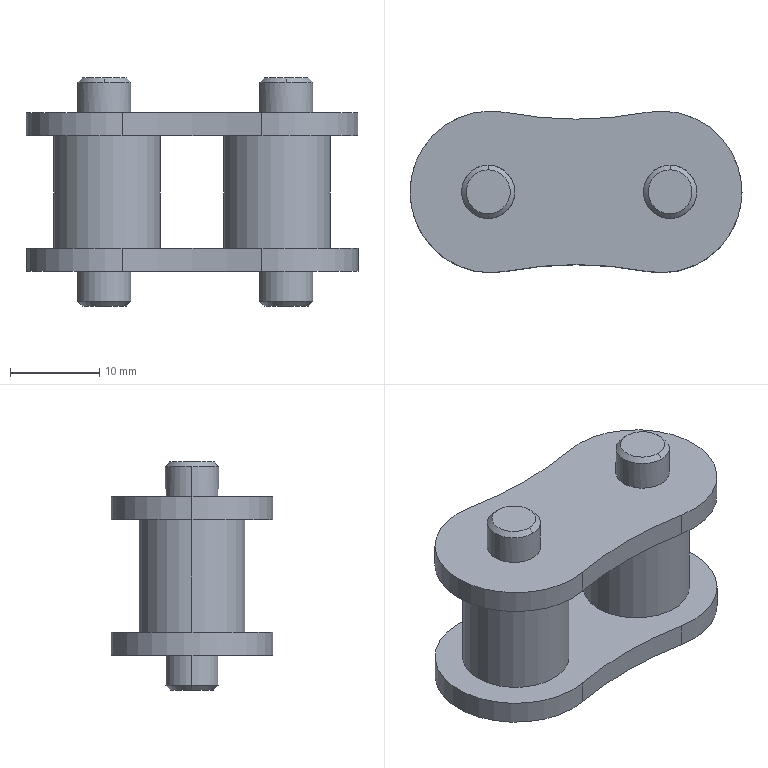Part | SolidWorks | features MoveFace 2, BaseBody 1 | 1 solid | 38 faces | box 37.13 x 18.08 x 25.52 mm | volume 6230 mm3 | cylinder 22 | cone 8 | plane 8 | commonest cylinder face diameters 5.96 x8 18.08 x6 11.91 x4 83.184 x4
STEP:
#1=CARTESIAN_POINT('',(-85.67,-121.776,-8.875));
#2=VERTEX_POINT('',#1);
#3=CARTESIAN_POINT('',(-96.411,-130.655,-8.875));
#4=VERTEX_POINT('',#3);
#5=CARTESIAN_POINT('',(-94.71,-121.776,-8.875));
#6=DIRECTION('',(0.,0.,-1.));
#7=DIRECTION('',(1.,0.,0.));
#8=AXIS2_PLACEMENT_3D('',#5,#6,#7);
#9=CIRCLE('',#8,9.04);
#10=EDGE_CURVE('',#2,#4,#9,.T.);
#11=ORIENTED_EDGE('',*,*,#10,.F.);
#12=CARTESIAN_POINT('',(-85.67,-121.776,-6.285));
#13=VERTEX_POINT('',#12);
#14=CARTESIAN_POINT('',(-85.67,-121.776,-8.875));
#15=DIRECTION('',(0.,0.,1.));
#16=VECTOR('',#15,1000.);
#17=LINE('',#14,#16);
#18=EDGE_CURVE('',#2,#13,#17,.T.);
#19=ORIENTED_EDGE('',*,*,#18,.T.);
#20=CARTESIAN_POINT('',(-96.411,-130.655,-6.285));
#21=VERTEX_POINT('',#20);
#22=CARTESIAN_POINT('',(-94.71,-121.776,-6.285));
#23=DIRECTION('',(0.,0.,-1.));
#24=DIRECTION('',(1.,0.,0.));
#25=AXIS2_PLACEMENT_3D('',#22,#23,#24);
#26=CIRCLE('',#25,9.04);
#27=EDGE_CURVE('',#13,#21,#26,.T.);
#28=ORIENTED_EDGE('',*,*,#27,.T.);
#29=CARTESIAN_POINT('',(-96.411,-130.655,-8.875));
#30=DIRECTION('',(0.,0.,-1.));
#31=VECTOR('',#30,1000.);
#32=LINE('',#29,#31);
#33=EDGE_CURVE('',#21,#4,#32,.T.);
#34=ORIENTED_EDGE('',*,*,#33,.T.);
#35=EDGE_LOOP('',(#11,#19,#28,#34));
#36=FACE_OUTER_BOUND('',#35,.T.);
#37=CARTESIAN_POINT('',(-94.71,-121.776,-8.875));
#38=DIRECTION('',(0.,0.,1.));
#39=DIRECTION('',(1.,0.,0.));
#40=AXIS2_PLACEMENT_3D('',#37,#38,#39);
#41=CYLINDRICAL_SURFACE('',#40,9.04);
#42=ADVANCED_FACE('',(#36),#41,.T.);
#43=CARTESIAN_POINT('',(-111.08,-121.776,-12.242));
#44=VERTEX_POINT('',#43);
#45=CARTESIAN_POINT('',(-117.04,-121.776,-12.242));
#46=VERTEX_POINT('',#45);
#47=CARTESIAN_POINT('',(-114.06,-121.776,-12.242));
#48=DIRECTION('',(0.,0.,1.));
#49=DIRECTION('',(1.,0.,0.));
#50=AXIS2_PLACEMENT_3D('',#47,#48,#49);
#51=CIRCLE('',#50,2.98);
#52=EDGE_CURVE('',#44,#46,#51,.T.);
#53=ORIENTED_EDGE('',*,*,#52,.T.);
#54=CARTESIAN_POINT('',(-117.04,-121.776,-8.875));
#55=VERTEX_POINT('',#54);
#56=CARTESIAN_POINT('',(-117.04,-121.776,-12.76));
#57=DIRECTION('',(0.,0.,1.));
#58=VECTOR('',#57,1000.);
#59=LINE('',#56,#58);
#60=EDGE_CURVE('',#46,#55,#59,.T.);
#61=ORIENTED_EDGE('',*,*,#60,.T.);
#62=CARTESIAN_POINT('',(-111.08,-121.776,-8.875));
#63=VERTEX_POINT('',#62);
#64=CARTESIAN_POINT('',(-114.06,-121.776,-8.875));
#65=DIRECTION('',(0.,0.,1.));
#66=DIRECTION('',(1.,0.,0.));
#67=AXIS2_PLACEMENT_3D('',#64,#65,#66);
#68=CIRCLE('',#67,2.98);
#69=EDGE_CURVE('',#63,#55,#68,.T.);
#70=ORIENTED_EDGE('',*,*,#69,.F.);
#71=CARTESIAN_POINT('',(-111.08,-121.776,-12.76));
#72=DIRECTION('',(0.,0.,1.));
#73=VECTOR('',#72,1000.);
#74=LINE('',#71,#73);
#75=EDGE_CURVE('',#44,#63,#74,.T.);
#76=ORIENTED_EDGE('',*,*,#75,.F.);
#77=EDGE_LOOP('',(#53,#61,#70,#76));
#78=FACE_OUTER_BOUND('',#77,.T.);
#79=CARTESIAN_POINT('',(-114.06,-121.776,-12.76));
#80=DIRECTION('',(0.,0.,1.));
#81=DIRECTION('',(1.,0.,0.));
#82=AXIS2_PLACEMENT_3D('',#79,#80,#81);
#83=CYLINDRICAL_SURFACE('',#82,2.98);
#84=ADVANCED_FACE('',(#78),#83,.T.);
#85=CARTESIAN_POINT('',(-90.73,-121.776,-12.242));
#86=VERTEX_POINT('',#85);
#87=CARTESIAN_POINT('',(-96.69,-121.776,-12.242));
#88=VERTEX_POINT('',#87);
#89=CARTESIAN_POINT('',(-93.71,-121.776,-12.242));
#90=DIRECTION('',(0.,0.,1.));
#91=DIRECTION('',(1.,0.,0.));
#92=AXIS2_PLACEMENT_3D('',#89,#90,#91);
#93=CIRCLE('',#92,2.98);
#94=EDGE_CURVE('',#86,#88,#93,.T.);
#95=ORIENTED_EDGE('',*,*,#94,.T.);
#96=CARTESIAN_POINT('',(-96.69,-121.776,-8.875));
#97=VERTEX_POINT('',#96);
#98=CARTESIAN_POINT('',(-96.69,-121.776,-12.76));
#99=DIRECTION('',(0.,0.,1.));
#100=VECTOR('',#99,1000.);
#101=LINE('',#98,#100);
#102=EDGE_CURVE('',#88,#97,#101,.T.);
#103=ORIENTED_EDGE('',*,*,#102,.T.);
#104=CARTESIAN_POINT('',(-90.73,-121.776,-8.875));
#105=VERTEX_POINT('',#104);
#106=CARTESIAN_POINT('',(-93.71,-121.776,-8.875));
#107=DIRECTION('',(0.,0.,1.));
#108=DIRECTION('',(1.,0.,0.));
#109=AXIS2_PLACEMENT_3D('',#106,#107,#108);
#110=CIRCLE('',#109,2.98);
#111=EDGE_CURVE('',#105,#97,#110,.T.);
#112=ORIENTED_EDGE('',*,*,#111,.F.);
#113=CARTESIAN_POINT('',(-90.73,-121.776,-12.76));
#114=DIRECTION('',(0.,0.,1.));
#115=VECTOR('',#114,1000.);
#116=LINE('',#113,#115);
#117=EDGE_CURVE('',#86,#105,#116,.T.);
#118=ORIENTED_EDGE('',*,*,#117,.F.);
#119=EDGE_LOOP('',(#95,#103,#112,#118));
#120=FACE_OUTER_BOUND('',#119,.T.);
#121=CARTESIAN_POINT('',(-93.71,-121.776,-12.76));
#122=DIRECTION('',(0.,0.,1.));
#123=DIRECTION('',(1.,0.,0.));
#124=AXIS2_PLACEMENT_3D('',#121,#122,#123);
#125=CYLINDRICAL_SURFACE('',#124,2.98);
#126=ADVANCED_FACE('',(#120),#125,.T.);
#127=CARTESIAN_POINT('',(-111.598,-121.776,-12.76));
#128=VERTEX_POINT('',#127);
#129=CARTESIAN_POINT('',(-116.522,-121.776,-12.76));
#130=VERTEX_POINT('',#129);
#131=CARTESIAN_POINT('',(-114.06,-121.776,-12.76));
#132=DIRECTION('',(0.,0.,1.));
#133=DIRECTION('',(1.,0.,0.));
#134=AXIS2_PLACEMENT_3D('',#131,#132,#133);
#135=CIRCLE('',#134,2.462);
#136=EDGE_CURVE('',#128,#130,#135,.T.);
#137=ORIENTED_EDGE('',*,*,#136,.T.);
#138=CARTESIAN_POINT('',(-117.04,-121.776,-12.242));
#139=DIRECTION('',(-0.7071,0.,0.7071));
#140=VECTOR('',#139,1000.);
#141=LINE('',#138,#140);
#142=EDGE_CURVE('',#130,#46,#141,.T.);
#143=ORIENTED_EDGE('',*,*,#142,.T.);
#144=ORIENTED_EDGE('',*,*,#52,.F.);
#145=CARTESIAN_POINT('',(-111.08,-121.776,-12.242));
#146=DIRECTION('',(0.7071,0.,0.7071));
#147=VECTOR('',#146,1000.);
#148=LINE('',#145,#147);
#149=EDGE_CURVE('',#128,#44,#148,.T.);
#150=ORIENTED_EDGE('',*,*,#149,.F.);
#151=EDGE_LOOP('',(#137,#143,#144,#150));
#152=FACE_OUTER_BOUND('',#151,.T.);
#153=CARTESIAN_POINT('',(-114.06,-121.776,-12.242));
#154=DIRECTION('',(0.,0.,1.));
#155=DIRECTION('',(1.,0.,0.));
#156=AXIS2_PLACEMENT_3D('',#153,#154,#155);
#157=CONICAL_SURFACE('',#156,2.98,0.7854);
#158=ADVANCED_FACE('',(#152),#157,.T.);
#159=CARTESIAN_POINT('',(-91.248,-121.776,-12.76));
#160=VERTEX_POINT('',#159);
#161=CARTESIAN_POINT('',(-96.172,-121.776,-12.76));
#162=VERTEX_POINT('',#161);
#163=CARTESIAN_POINT('',(-93.71,-121.776,-12.76));
#164=DIRECTION('',(0.,0.,1.));
#165=DIRECTION('',(1.,0.,0.));
#166=AXIS2_PLACEMENT_3D('',#163,#164,#165);
#167=CIRCLE('',#166,2.462);
#168=EDGE_CURVE('',#160,#162,#167,.T.);
#169=ORIENTED_EDGE('',*,*,#168,.T.);
#170=CARTESIAN_POINT('',(-96.69,-121.776,-12.242));
#171=DIRECTION('',(-0.7071,0.,0.7071));
#172=VECTOR('',#171,1000.);
#173=LINE('',#170,#172);
#174=EDGE_CURVE('',#162,#88,#173,.T.);
#175=ORIENTED_EDGE('',*,*,#174,.T.);
#176=ORIENTED_EDGE('',*,*,#94,.F.);
#177=CARTESIAN_POINT('',(-90.73,-121.776,-12.242));
#178=DIRECTION('',(0.7071,0.,0.7071));
#179=VECTOR('',#178,1000.);
#180=LINE('',#177,#179);
#181=EDGE_CURVE('',#160,#86,#180,.T.);
#182=ORIENTED_EDGE('',*,*,#181,.F.);
#183=EDGE_LOOP('',(#169,#175,#176,#182));
#184=FACE_OUTER_BOUND('',#183,.T.);
#185=CARTESIAN_POINT('',(-93.71,-121.776,-12.242));
#186=DIRECTION('',(0.,0.,1.));
#187=DIRECTION('',(1.,0.,0.));
#188=AXIS2_PLACEMENT_3D('',#185,#186,#187);
#189=CONICAL_SURFACE('',#188,2.98,0.7854);
#190=ADVANCED_FACE('',(#184),#189,.T.);
#191=CARTESIAN_POINT('',(-119.715,-121.776,6.285));
#192=VERTEX_POINT('',#191);
#193=CARTESIAN_POINT('',(-107.805,-121.776,6.285));
#194=VERTEX_POINT('',#193);
#195=CARTESIAN_POINT('',(-113.76,-121.776,6.285));
#196=DIRECTION('',(0.,0.,-1.));
#197=DIRECTION('',(-1.,0.,0.));
#198=AXIS2_PLACEMENT_3D('',#195,#196,#197);
#199=CIRCLE('',#198,5.955);
#200=EDGE_CURVE('',#192,#194,#199,.T.);
#201=ORIENTED_EDGE('',*,*,#200,.T.);
#202=CARTESIAN_POINT('',(-107.805,-121.776,-6.285));
#203=VERTEX_POINT('',#202);
#204=CARTESIAN_POINT('',(-107.805,-121.776,6.285));
#205=DIRECTION('',(0.,0.,-1.));
#206=VECTOR('',#205,1000.);
#207=LINE('',#204,#206);
#208=EDGE_CURVE('',#194,#203,#207,.T.);
#209=ORIENTED_EDGE('',*,*,#208,.T.);
#210=CARTESIAN_POINT('',(-119.715,-121.776,-6.285));
#211=VERTEX_POINT('',#210);
#212=CARTESIAN_POINT('',(-113.76,-121.776,-6.285));
#213=DIRECTION('',(0.,0.,1.));
#214=DIRECTION('',(-1.,0.,0.));
#215=AXIS2_PLACEMENT_3D('',#212,#213,#214);
#216=CIRCLE('',#215,5.955);
#217=EDGE_CURVE('',#203,#211,#216,.T.);
#218=ORIENTED_EDGE('',*,*,#217,.T.);
#219=CARTESIAN_POINT('',(-119.715,-121.776,6.285));
#220=DIRECTION('',(0.,0.,-1.));
#221=VECTOR('',#220,1000.);
#222=LINE('',#219,#221);
#223=EDGE_CURVE('',#192,#211,#222,.T.);
#224=ORIENTED_EDGE('',*,*,#223,.F.);
#225=EDGE_LOOP('',(#201,#209,#218,#224));
#226=FACE_OUTER_BOUND('',#225,.T.);
#227=CARTESIAN_POINT('',(-113.76,-121.776,6.285));
#228=DIRECTION('',(0.,0.,-1.));
#229=DIRECTION('',(-1.,0.,0.));
#230=AXIS2_PLACEMENT_3D('',#227,#228,#229);
#231=CYLINDRICAL_SURFACE('',#230,5.955);
#232=ADVANCED_FACE('',(#226),#231,.T.);
#233=CARTESIAN_POINT('',(-100.665,-121.776,6.285));
#234=VERTEX_POINT('',#233);
#235=CARTESIAN_POINT('',(-88.755,-121.776,6.285));
#236=VERTEX_POINT('',#235);
#237=CARTESIAN_POINT('',(-94.71,-121.776,6.285));
#238=DIRECTION('',(0.,0.,-1.));
#239=DIRECTION('',(-1.,0.,0.));
#240=AXIS2_PLACEMENT_3D('',#237,#238,#239);
#241=CIRCLE('',#240,5.955);
#242=EDGE_CURVE('',#234,#236,#241,.T.);
#243=ORIENTED_EDGE('',*,*,#242,.T.);
#244=CARTESIAN_POINT('',(-88.755,-121.776,-6.285));
#245=VERTEX_POINT('',#244);
#246=CARTESIAN_POINT('',(-88.755,-121.776,6.285));
#247=DIRECTION('',(0.,0.,-1.));
#248=VECTOR('',#247,1000.);
#249=LINE('',#246,#248);
#250=EDGE_CURVE('',#236,#245,#249,.T.);
#251=ORIENTED_EDGE('',*,*,#250,.T.);
#252=CARTESIAN_POINT('',(-100.665,-121.776,-6.285));
#253=VERTEX_POINT('',#252);
#254=CARTESIAN_POINT('',(-94.71,-121.776,-6.285));
#255=DIRECTION('',(0.,0.,1.));
#256=DIRECTION('',(-1.,0.,0.));
#257=AXIS2_PLACEMENT_3D('',#254,#255,#256);
#258=CIRCLE('',#257,5.955);
#259=EDGE_CURVE('',#245,#253,#258,.T.);
#260=ORIENTED_EDGE('',*,*,#259,.T.);
#261=CARTESIAN_POINT('',(-100.665,-121.776,6.285));
#262=DIRECTION('',(0.,0.,-1.));
#263=VECTOR('',#262,1000.);
#264=LINE('',#261,#263);
#265=EDGE_CURVE('',#234,#253,#264,.T.);
#266=ORIENTED_EDGE('',*,*,#265,.F.);
#267=EDGE_LOOP('',(#243,#251,#260,#266));
#268=FACE_OUTER_BOUND('',#267,.T.);
#269=CARTESIAN_POINT('',(-94.71,-121.776,6.285));
#270=DIRECTION('',(0.,0.,-1.));
#271=DIRECTION('',(-1.,0.,0.));
#272=AXIS2_PLACEMENT_3D('',#269,#270,#271);
#273=CYLINDRICAL_SURFACE('',#272,5.955);
#274=ADVANCED_FACE('',(#268),#273,.T.);
#275=CARTESIAN_POINT('',(-112.06,-130.655,8.875));
#276=VERTEX_POINT('',#275);
#277=CARTESIAN_POINT('',(-122.8,-121.776,8.875));
#278=VERTEX_POINT('',#277);
#279=CARTESIAN_POINT('',(-113.76,-121.776,8.875));
#280=DIRECTION('',(0.,0.,-1.));
#281=DIRECTION('',(-1.,0.,0.));
#282=AXIS2_PLACEMENT_3D('',#279,#280,#281);
#283=CIRCLE('',#282,9.04);
#284=EDGE_CURVE('',#276,#278,#283,.T.);
#285=ORIENTED_EDGE('',*,*,#284,.T.);
#286=CARTESIAN_POINT('',(-122.8,-121.776,6.285));
#287=VERTEX_POINT('',#286);
#288=CARTESIAN_POINT('',(-122.8,-121.776,8.875));
#289=DIRECTION('',(0.,0.,-1.));
#290=VECTOR('',#289,1000.);
#291=LINE('',#288,#290);
#292=EDGE_CURVE('',#278,#287,#291,.T.);
#293=ORIENTED_EDGE('',*,*,#292,.T.);
#294=CARTESIAN_POINT('',(-112.06,-130.655,6.285));
#295=VERTEX_POINT('',#294);
#296=CARTESIAN_POINT('',(-113.76,-121.776,6.285));
#297=DIRECTION('',(0.,0.,1.));
#298=DIRECTION('',(-1.,0.,0.));
#299=AXIS2_PLACEMENT_3D('',#296,#297,#298);
#300=CIRCLE('',#299,9.04);
#301=EDGE_CURVE('',#287,#295,#300,.T.);
#302=ORIENTED_EDGE('',*,*,#301,.T.);
#303=CARTESIAN_POINT('',(-112.06,-130.655,8.875));
#304=DIRECTION('',(0.,0.,1.));
#305=VECTOR('',#304,1000.);
#306=LINE('',#303,#305);
#307=EDGE_CURVE('',#295,#276,#306,.T.);
#308=ORIENTED_EDGE('',*,*,#307,.T.);
#309=EDGE_LOOP('',(#285,#293,#302,#308));
#310=FACE_OUTER_BOUND('',#309,.T.);
#311=CARTESIAN_POINT('',(-113.76,-121.776,8.875));
#312=DIRECTION('',(0.,0.,-1.));
#313=DIRECTION('',(-1.,0.,0.));
#314=AXIS2_PLACEMENT_3D('',#311,#312,#313);
#315=CYLINDRICAL_SURFACE('',#314,9.04);
#316=ADVANCED_FACE('',(#310),#315,.T.);
#317=CARTESIAN_POINT('',(-93.71,-118.796,12.242));
#318=VERTEX_POINT('',#317);
#319=CARTESIAN_POINT('',(-90.73,-121.776,12.242));
#320=VERTEX_POINT('',#319);
#321=CARTESIAN_POINT('',(-93.71,-121.776,12.242));
#322=DIRECTION('',(0.,0.,-1.));
#323=DIRECTION('',(-1.,0.,0.));
#324=AXIS2_PLACEMENT_3D('',#321,#322,#323);
#325=CIRCLE('',#324,2.98);
#326=EDGE_CURVE('',#318,#320,#325,.T.);
#327=ORIENTED_EDGE('',*,*,#326,.T.);
#328=CARTESIAN_POINT('',(-90.73,-121.776,8.875));
#329=VERTEX_POINT('',#328);
#330=CARTESIAN_POINT('',(-90.73,-121.776,12.76));
#331=DIRECTION('',(0.,0.,-1.));
#332=VECTOR('',#331,1000.);
#333=LINE('',#330,#332);
#334=EDGE_CURVE('',#320,#329,#333,.T.);
#335=ORIENTED_EDGE('',*,*,#334,.T.);
#336=CARTESIAN_POINT('',(-96.69,-121.776,8.875));
#337=VERTEX_POINT('',#336);
#338=CARTESIAN_POINT('',(-93.71,-121.776,8.875));
#339=DIRECTION('',(0.,0.,-1.));
#340=DIRECTION('',(-1.,0.,0.));
#341=AXIS2_PLACEMENT_3D('',#338,#339,#340);
#342=CIRCLE('',#341,2.98);
#343=EDGE_CURVE('',#337,#329,#342,.T.);
#344=ORIENTED_EDGE('',*,*,#343,.F.);
#345=CARTESIAN_POINT('',(-96.69,-121.776,12.242));
#346=VERTEX_POINT('',#345);
#347=CARTESIAN_POINT('',(-96.69,-121.776,12.76));
#348=DIRECTION('',(0.,0.,-1.));
#349=VECTOR('',#348,1000.);
#350=LINE('',#347,#349);
#351=EDGE_CURVE('',#346,#337,#350,.T.);
#352=ORIENTED_EDGE('',*,*,#351,.F.);
#353=CARTESIAN_POINT('',(-93.71,-121.776,12.242));
#354=DIRECTION('',(0.,0.,-1.));
#355=DIRECTION('',(-1.,0.,0.));
#356=AXIS2_PLACEMENT_3D('',#353,#354,#355);
#357=CIRCLE('',#356,2.98);
#358=EDGE_CURVE('',#346,#318,#357,.T.);
#359=ORIENTED_EDGE('',*,*,#358,.T.);
#360=EDGE_LOOP('',(#327,#335,#344,#352,#359));
#361=FACE_OUTER_BOUND('',#360,.T.);
#362=CARTESIAN_POINT('',(-93.71,-121.776,12.76));
#363=DIRECTION('',(0.,0.,-1.));
#364=DIRECTION('',(-1.,0.,0.));
#365=AXIS2_PLACEMENT_3D('',#362,#363,#364);
#366=CYLINDRICAL_SURFACE('',#365,2.98);
#367=ADVANCED_FACE('',(#361),#366,.T.);
#368=CARTESIAN_POINT('',(-114.06,-118.796,12.242));
#369=VERTEX_POINT('',#368);
#370=CARTESIAN_POINT('',(-111.08,-121.776,12.242));
#371=VERTEX_POINT('',#370);
#372=CARTESIAN_POINT('',(-114.06,-121.776,12.242));
#373=DIRECTION('',(0.,0.,-1.));
#374=DIRECTION('',(-1.,0.,0.));
#375=AXIS2_PLACEMENT_3D('',#372,#373,#374);
#376=CIRCLE('',#375,2.98);
#377=EDGE_CURVE('',#369,#371,#376,.T.);
#378=ORIENTED_EDGE('',*,*,#377,.T.);
#379=CARTESIAN_POINT('',(-111.08,-121.776,8.875));
#380=VERTEX_POINT('',#379);
#381=CARTESIAN_POINT('',(-111.08,-121.776,12.76));
#382=DIRECTION('',(0.,0.,-1.));
#383=VECTOR('',#382,1000.);
#384=LINE('',#381,#383);
#385=EDGE_CURVE('',#371,#380,#384,.T.);
#386=ORIENTED_EDGE('',*,*,#385,.T.);
#387=CARTESIAN_POINT('',(-117.04,-121.776,8.875));
#388=VERTEX_POINT('',#387);
#389=CARTESIAN_POINT('',(-114.06,-121.776,8.875));
#390=DIRECTION('',(0.,0.,-1.));
#391=DIRECTION('',(-1.,0.,0.));
#392=AXIS2_PLACEMENT_3D('',#389,#390,#391);
#393=CIRCLE('',#392,2.98);
#394=EDGE_CURVE('',#388,#380,#393,.T.);
#395=ORIENTED_EDGE('',*,*,#394,.F.);
#396=CARTESIAN_POINT('',(-117.04,-121.776,12.242));
#397=VERTEX_POINT('',#396);
#398=CARTESIAN_POINT('',(-117.04,-121.776,12.76));
#399=DIRECTION('',(0.,0.,-1.));
#400=VECTOR('',#399,1000.);
#401=LINE('',#398,#400);
#402=EDGE_CURVE('',#397,#388,#401,.T.);
#403=ORIENTED_EDGE('',*,*,#402,.F.);
#404=CARTESIAN_POINT('',(-114.06,-121.776,12.242));
#405=DIRECTION('',(0.,0.,-1.));
#406=DIRECTION('',(-1.,0.,0.));
#407=AXIS2_PLACEMENT_3D('',#404,#405,#406);
#408=CIRCLE('',#407,2.98);
#409=EDGE_CURVE('',#397,#369,#408,.T.);
#410=ORIENTED_EDGE('',*,*,#409,.T.);
#411=EDGE_LOOP('',(#378,#386,#395,#403,#410));
#412=FACE_OUTER_BOUND('',#411,.T.);
#413=CARTESIAN_POINT('',(-114.06,-121.776,12.76));
#414=DIRECTION('',(0.,0.,-1.));
#415=DIRECTION('',(-1.,0.,0.));
#416=AXIS2_PLACEMENT_3D('',#413,#414,#415);
#417=CYLINDRICAL_SURFACE('',#416,2.98);
#418=ADVANCED_FACE('',(#412),#417,.T.);
#419=CARTESIAN_POINT('',(-93.71,-119.314,12.76));
#420=VERTEX_POINT('',#419);
#421=CARTESIAN_POINT('',(-93.71,-124.238,12.76));
#422=VERTEX_POINT('',#421);
#423=CARTESIAN_POINT('',(-93.71,-121.776,12.76));
#424=DIRECTION('',(0.,0.,-1.));
#425=DIRECTION('',(0.,1.,0.));
#426=AXIS2_PLACEMENT_3D('',#423,#424,#425);
#427=CIRCLE('',#426,2.462);
#428=EDGE_CURVE('',#420,#422,#427,.T.);
#429=ORIENTED_EDGE('',*,*,#428,.T.);
#430=CARTESIAN_POINT('',(-93.71,-124.756,12.242));
#431=VERTEX_POINT('',#430);
#432=CARTESIAN_POINT('',(-93.71,-124.756,12.242));
#433=DIRECTION('',(0.,-0.7071,-0.7071));
#434=VECTOR('',#433,1000.);
#435=LINE('',#432,#434);
#436=EDGE_CURVE('',#422,#431,#435,.T.);
#437=ORIENTED_EDGE('',*,*,#436,.T.);
#438=CARTESIAN_POINT('',(-93.71,-121.776,12.242));
#439=DIRECTION('',(0.,0.,-1.));
#440=DIRECTION('',(-1.,0.,0.));
#441=AXIS2_PLACEMENT_3D('',#438,#439,#440);
#442=CIRCLE('',#441,2.98);
#443=EDGE_CURVE('',#320,#431,#442,.T.);
#444=ORIENTED_EDGE('',*,*,#443,.F.);
#445=ORIENTED_EDGE('',*,*,#326,.F.);
#446=CARTESIAN_POINT('',(-93.71,-118.796,12.242));
#447=DIRECTION('',(0.,0.7071,-0.7071));
#448=VECTOR('',#447,1000.);
#449=LINE('',#446,#448);
#450=EDGE_CURVE('',#420,#318,#449,.T.);
#451=ORIENTED_EDGE('',*,*,#450,.F.);
#452=EDGE_LOOP('',(#429,#437,#444,#445,#451));
#453=FACE_OUTER_BOUND('',#452,.T.);
#454=CARTESIAN_POINT('',(-93.71,-121.776,12.242));
#455=DIRECTION('',(0.,0.,-1.));
#456=DIRECTION('',(0.,1.,0.));
#457=AXIS2_PLACEMENT_3D('',#454,#455,#456);
#458=CONICAL_SURFACE('',#457,2.98,0.7854);
#459=ADVANCED_FACE('',(#453),#458,.T.);
#460=CARTESIAN_POINT('',(-114.06,-119.314,12.76));
#461=VERTEX_POINT('',#460);
#462=CARTESIAN_POINT('',(-114.06,-124.238,12.76));
#463=VERTEX_POINT('',#462);
#464=CARTESIAN_POINT('',(-114.06,-121.776,12.76));
#465=DIRECTION('',(0.,0.,-1.));
#466=DIRECTION('',(0.,1.,0.));
#467=AXIS2_PLACEMENT_3D('',#464,#465,#466);
#468=CIRCLE('',#467,2.462);
#469=EDGE_CURVE('',#461,#463,#468,.T.);
#470=ORIENTED_EDGE('',*,*,#469,.T.);
#471=CARTESIAN_POINT('',(-114.06,-124.756,12.242));
#472=VERTEX_POINT('',#471);
#473=CARTESIAN_POINT('',(-114.06,-124.756,12.242));
#474=DIRECTION('',(0.,-0.7071,-0.7071));
#475=VECTOR('',#474,1000.);
#476=LINE('',#473,#475);
#477=EDGE_CURVE('',#463,#472,#476,.T.);
#478=ORIENTED_EDGE('',*,*,#477,.T.);
#479=CARTESIAN_POINT('',(-114.06,-121.776,12.242));
#480=DIRECTION('',(0.,0.,-1.));
#481=DIRECTION('',(-1.,0.,0.));
#482=AXIS2_PLACEMENT_3D('',#479,#480,#481);
#483=CIRCLE('',#482,2.98);
#484=EDGE_CURVE('',#371,#472,#483,.T.);
#485=ORIENTED_EDGE('',*,*,#484,.F.);
#486=ORIENTED_EDGE('',*,*,#377,.F.);
#487=CARTESIAN_POINT('',(-114.06,-118.796,12.242));
#488=DIRECTION('',(0.,0.7071,-0.7071));
#489=VECTOR('',#488,1000.);
#490=LINE('',#487,#489);
#491=EDGE_CURVE('',#461,#369,#490,.T.);
#492=ORIENTED_EDGE('',*,*,#491,.F.);
#493=EDGE_LOOP('',(#470,#478,#485,#486,#492));
#494=FACE_OUTER_BOUND('',#493,.T.);
#495=CARTESIAN_POINT('',(-114.06,-121.776,12.242));
#496=DIRECTION('',(0.,0.,-1.));
#497=DIRECTION('',(0.,1.,0.));
#498=AXIS2_PLACEMENT_3D('',#495,#496,#497);
#499=CONICAL_SURFACE('',#498,2.98,0.7854);
#500=ADVANCED_FACE('',(#494),#499,.T.);
#501=CARTESIAN_POINT('',(-112.06,-130.655,-8.875));
#502=VERTEX_POINT('',#501);
#503=CARTESIAN_POINT('',(-112.06,-112.897,-8.875));
#504=VERTEX_POINT('',#503);
#505=CARTESIAN_POINT('',(-113.76,-121.776,-8.875));
#506=DIRECTION('',(0.,0.,-1.));
#507=DIRECTION('',(1.,0.,0.));
#508=AXIS2_PLACEMENT_3D('',#505,#506,#507);
#509=CIRCLE('',#508,9.04);
#510=EDGE_CURVE('',#502,#504,#509,.T.);
#511=ORIENTED_EDGE('',*,*,#510,.T.);
#512=CARTESIAN_POINT('',(-96.411,-112.897,-8.875));
#513=VERTEX_POINT('',#512);
#514=CARTESIAN_POINT('',(-104.235,-72.048,-8.875));
#515=DIRECTION('',(0.,0.,1.));
#516=DIRECTION('',(1.,0.,0.));
#517=AXIS2_PLACEMENT_3D('',#514,#515,#516);
#518=CIRCLE('',#517,41.592);
#519=EDGE_CURVE('',#504,#513,#518,.T.);
#520=ORIENTED_EDGE('',*,*,#519,.T.);
#521=CARTESIAN_POINT('',(-94.71,-121.776,-8.875));
#522=DIRECTION('',(0.,0.,-1.));
#523=DIRECTION('',(1.,0.,0.));
#524=AXIS2_PLACEMENT_3D('',#521,#522,#523);
#525=CIRCLE('',#524,9.04);
#526=EDGE_CURVE('',#513,#2,#525,.T.);
#527=ORIENTED_EDGE('',*,*,#526,.T.);
#528=ORIENTED_EDGE('',*,*,#10,.T.);
#529=CARTESIAN_POINT('',(-104.235,-171.504,-8.875));
#530=DIRECTION('',(0.,0.,1.));
#531=DIRECTION('',(1.,0.,0.));
#532=AXIS2_PLACEMENT_3D('',#529,#530,#531);
#533=CIRCLE('',#532,41.592);
#534=EDGE_CURVE('',#4,#502,#533,.T.);
#535=ORIENTED_EDGE('',*,*,#534,.T.);
#536=EDGE_LOOP('',(#511,#520,#527,#528,#535));
#537=FACE_OUTER_BOUND('',#536,.T.);
#538=ORIENTED_EDGE('',*,*,#69,.T.);
#539=CARTESIAN_POINT('',(-114.06,-121.776,-8.875));
#540=DIRECTION('',(0.,0.,1.));
#541=DIRECTION('',(1.,0.,0.));
#542=AXIS2_PLACEMENT_3D('',#539,#540,#541);
#543=CIRCLE('',#542,2.98);
#544=EDGE_CURVE('',#55,#63,#543,.T.);
#545=ORIENTED_EDGE('',*,*,#544,.T.);
#546=EDGE_LOOP('',(#538,#545));
#547=FACE_BOUND('',#546,.T.);
#548=ORIENTED_EDGE('',*,*,#111,.T.);
#549=CARTESIAN_POINT('',(-93.71,-121.776,-8.875));
#550=DIRECTION('',(0.,0.,1.));
#551=DIRECTION('',(1.,0.,0.));
#552=AXIS2_PLACEMENT_3D('',#549,#550,#551);
#553=CIRCLE('',#552,2.98);
#554=EDGE_CURVE('',#97,#105,#553,.T.);
#555=ORIENTED_EDGE('',*,*,#554,.T.);
#556=EDGE_LOOP('',(#548,#555));
#557=FACE_BOUND('',#556,.T.);
#558=CARTESIAN_POINT('',(-99.473,-96.912,-8.875));
#559=DIRECTION('',(0.,0.,-1.));
#560=DIRECTION('',(-1.,0.,0.));
#561=AXIS2_PLACEMENT_3D('',#558,#559,#560);
#562=PLANE('',#561);
#563=ADVANCED_FACE('',(#537,#547,#557),#562,.T.);
#564=CARTESIAN_POINT('',(-112.06,-130.655,-6.285));
#565=VERTEX_POINT('',#564);
#566=CARTESIAN_POINT('',(-112.06,-112.897,-6.285));
#567=VERTEX_POINT('',#566);
#568=CARTESIAN_POINT('',(-113.76,-121.776,-6.285));
#569=DIRECTION('',(0.,0.,-1.));
#570=DIRECTION('',(1.,0.,0.));
#571=AXIS2_PLACEMENT_3D('',#568,#569,#570);
#572=CIRCLE('',#571,9.04);
#573=EDGE_CURVE('',#565,#567,#572,.T.);
#574=ORIENTED_EDGE('',*,*,#573,.T.);
#575=CARTESIAN_POINT('',(-112.06,-112.897,-8.875));
#576=DIRECTION('',(0.,0.,-1.));
#577=VECTOR('',#576,1000.);
#578=LINE('',#575,#577);
#579=EDGE_CURVE('',#567,#504,#578,.T.);
#580=ORIENTED_EDGE('',*,*,#579,.T.);
#581=ORIENTED_EDGE('',*,*,#510,.F.);
#582=CARTESIAN_POINT('',(-112.06,-130.655,-8.875));
#583=DIRECTION('',(0.,0.,1.));
#584=VECTOR('',#583,1000.);
#585=LINE('',#582,#584);
#586=EDGE_CURVE('',#502,#565,#585,.T.);
#587=ORIENTED_EDGE('',*,*,#586,.T.);
#588=EDGE_LOOP('',(#574,#580,#581,#587));
#589=FACE_OUTER_BOUND('',#588,.T.);
#590=CARTESIAN_POINT('',(-113.76,-121.776,-8.875));
#591=DIRECTION('',(0.,0.,1.));
#592=DIRECTION('',(1.,0.,0.));
#593=AXIS2_PLACEMENT_3D('',#590,#591,#592);
#594=CYLINDRICAL_SURFACE('',#593,9.04);
#595=ADVANCED_FACE('',(#589),#594,.T.);
#596=ORIENTED_EDGE('',*,*,#586,.F.);
#597=ORIENTED_EDGE('',*,*,#534,.F.);
#598=ORIENTED_EDGE('',*,*,#33,.F.);
#599=CARTESIAN_POINT('',(-104.235,-171.504,-6.285));
#600=DIRECTION('',(0.,0.,-1.));
#601=DIRECTION('',(1.,0.,0.));
#602=AXIS2_PLACEMENT_3D('',#599,#600,#601);
#603=CIRCLE('',#602,41.592);
#604=EDGE_CURVE('',#565,#21,#603,.T.);
#605=ORIENTED_EDGE('',*,*,#604,.F.);
#606=EDGE_LOOP('',(#596,#597,#598,#605));
#607=FACE_OUTER_BOUND('',#606,.T.);
#608=CARTESIAN_POINT('',(-104.235,-171.504,-8.875));
#609=DIRECTION('',(0.,0.,1.));
#610=DIRECTION('',(1.,0.,0.));
#611=AXIS2_PLACEMENT_3D('',#608,#609,#610);
#612=CYLINDRICAL_SURFACE('',#611,41.592);
#613=ADVANCED_FACE('',(#607),#612,.F.);
#614=ORIENTED_EDGE('',*,*,#18,.F.);
#615=ORIENTED_EDGE('',*,*,#526,.F.);
#616=CARTESIAN_POINT('',(-96.411,-112.897,-6.285));
#617=VERTEX_POINT('',#616);
#618=CARTESIAN_POINT('',(-96.411,-112.897,-8.875));
#619=DIRECTION('',(0.,0.,1.));
#620=VECTOR('',#619,1000.);
#621=LINE('',#618,#620);
#622=EDGE_CURVE('',#513,#617,#621,.T.);
#623=ORIENTED_EDGE('',*,*,#622,.T.);
#624=CARTESIAN_POINT('',(-94.71,-121.776,-6.285));
#625=DIRECTION('',(0.,0.,-1.));
#626=DIRECTION('',(1.,0.,0.));
#627=AXIS2_PLACEMENT_3D('',#624,#625,#626);
#628=CIRCLE('',#627,9.04);
#629=EDGE_CURVE('',#617,#13,#628,.T.);
#630=ORIENTED_EDGE('',*,*,#629,.T.);
#631=EDGE_LOOP('',(#614,#615,#623,#630));
#632=FACE_OUTER_BOUND('',#631,.T.);
#633=CARTESIAN_POINT('',(-94.71,-121.776,-8.875));
#634=DIRECTION('',(0.,0.,1.));
#635=DIRECTION('',(1.,0.,0.));
#636=AXIS2_PLACEMENT_3D('',#633,#634,#635);
#637=CYLINDRICAL_SURFACE('',#636,9.04);
#638=ADVANCED_FACE('',(#632),#637,.T.);
#639=ORIENTED_EDGE('',*,*,#622,.F.);
#640=ORIENTED_EDGE('',*,*,#519,.F.);
#641=ORIENTED_EDGE('',*,*,#579,.F.);
#642=CARTESIAN_POINT('',(-104.235,-72.048,-6.285));
#643=DIRECTION('',(0.,0.,-1.));
#644=DIRECTION('',(1.,0.,0.));
#645=AXIS2_PLACEMENT_3D('',#642,#643,#644);
#646=CIRCLE('',#645,41.592);
#647=EDGE_CURVE('',#617,#567,#646,.T.);
#648=ORIENTED_EDGE('',*,*,#647,.F.);
#649=EDGE_LOOP('',(#639,#640,#641,#648));
#650=FACE_OUTER_BOUND('',#649,.T.);
#651=CARTESIAN_POINT('',(-104.235,-72.048,-8.875));
#652=DIRECTION('',(0.,0.,1.));
#653=DIRECTION('',(1.,0.,0.));
#654=AXIS2_PLACEMENT_3D('',#651,#652,#653);
#655=CYLINDRICAL_SURFACE('',#654,41.592);
#656=ADVANCED_FACE('',(#650),#655,.F.);
#657=ORIENTED_EDGE('',*,*,#60,.F.);
#658=CARTESIAN_POINT('',(-114.06,-121.776,-12.242));
#659=DIRECTION('',(0.,0.,1.));
#660=DIRECTION('',(1.,0.,0.));
#661=AXIS2_PLACEMENT_3D('',#658,#659,#660);
#662=CIRCLE('',#661,2.98);
#663=EDGE_CURVE('',#46,#44,#662,.T.);
#664=ORIENTED_EDGE('',*,*,#663,.T.);
#665=ORIENTED_EDGE('',*,*,#75,.T.);
#666=ORIENTED_EDGE('',*,*,#544,.F.);
#667=EDGE_LOOP('',(#657,#664,#665,#666));
#668=FACE_OUTER_BOUND('',#667,.T.);
#669=CARTESIAN_POINT('',(-114.06,-121.776,-12.76));
#670=DIRECTION('',(0.,0.,1.));
#671=DIRECTION('',(1.,0.,0.));
#672=AXIS2_PLACEMENT_3D('',#669,#670,#671);
#673=CYLINDRICAL_SURFACE('',#672,2.98);
#674=ADVANCED_FACE('',(#668),#673,.T.);
#675=ORIENTED_EDGE('',*,*,#102,.F.);
#676=CARTESIAN_POINT('',(-93.71,-121.776,-12.242));
#677=DIRECTION('',(0.,0.,1.));
#678=DIRECTION('',(1.,0.,0.));
#679=AXIS2_PLACEMENT_3D('',#676,#677,#678);
#680=CIRCLE('',#679,2.98);
#681=EDGE_CURVE('',#88,#86,#680,.T.);
#682=ORIENTED_EDGE('',*,*,#681,.T.);
#683=ORIENTED_EDGE('',*,*,#117,.T.);
#684=ORIENTED_EDGE('',*,*,#554,.F.);
#685=EDGE_LOOP('',(#675,#682,#683,#684));
#686=FACE_OUTER_BOUND('',#685,.T.);
#687=CARTESIAN_POINT('',(-93.71,-121.776,-12.76));
#688=DIRECTION('',(0.,0.,1.));
#689=DIRECTION('',(1.,0.,0.));
#690=AXIS2_PLACEMENT_3D('',#687,#688,#689);
#691=CYLINDRICAL_SURFACE('',#690,2.98);
#692=ADVANCED_FACE('',(#686),#691,.T.);
#693=CARTESIAN_POINT('',(-113.76,-121.776,-6.285));
#694=DIRECTION('',(0.,0.,1.));
#695=DIRECTION('',(-1.,0.,0.));
#696=AXIS2_PLACEMENT_3D('',#693,#694,#695);
#697=CIRCLE('',#696,5.955);
#698=EDGE_CURVE('',#211,#203,#697,.T.);
#699=ORIENTED_EDGE('',*,*,#698,.F.);
#700=ORIENTED_EDGE('',*,*,#217,.F.);
#701=EDGE_LOOP('',(#699,#700));
#702=FACE_BOUND('',#701,.T.);
#703=ORIENTED_EDGE('',*,*,#573,.F.);
#704=ORIENTED_EDGE('',*,*,#604,.T.);
#705=ORIENTED_EDGE('',*,*,#27,.F.);
#706=ORIENTED_EDGE('',*,*,#629,.F.);
#707=ORIENTED_EDGE('',*,*,#647,.T.);
#708=EDGE_LOOP('',(#703,#704,#705,#706,#707));
#709=FACE_OUTER_BOUND('',#708,.T.);
#710=CARTESIAN_POINT('',(-94.71,-121.776,-6.285));
#711=DIRECTION('',(0.,0.,1.));
#712=DIRECTION('',(-1.,0.,0.));
#713=AXIS2_PLACEMENT_3D('',#710,#711,#712);
#714=CIRCLE('',#713,5.955);
#715=EDGE_CURVE('',#253,#245,#714,.T.);
#716=ORIENTED_EDGE('',*,*,#715,.F.);
#717=ORIENTED_EDGE('',*,*,#259,.F.);
#718=EDGE_LOOP('',(#716,#717));
#719=FACE_BOUND('',#718,.T.);
#720=CARTESIAN_POINT('',(-99.473,-96.912,-6.285));
#721=DIRECTION('',(0.,0.,-1.));
#722=DIRECTION('',(-1.,0.,0.));
#723=AXIS2_PLACEMENT_3D('',#720,#721,#722);
#724=PLANE('',#723);
#725=ADVANCED_FACE('',(#702,#709,#719),#724,.F.);
#726=ORIENTED_EDGE('',*,*,#142,.F.);
#727=CARTESIAN_POINT('',(-114.06,-121.776,-12.76));
#728=DIRECTION('',(0.,0.,1.));
#729=DIRECTION('',(1.,0.,0.));
#730=AXIS2_PLACEMENT_3D('',#727,#728,#729);
#731=CIRCLE('',#730,2.462);
#732=EDGE_CURVE('',#130,#128,#731,.T.);
#733=ORIENTED_EDGE('',*,*,#732,.T.);
#734=ORIENTED_EDGE('',*,*,#149,.T.);
#735=ORIENTED_EDGE('',*,*,#663,.F.);
#736=EDGE_LOOP('',(#726,#733,#734,#735));
#737=FACE_OUTER_BOUND('',#736,.T.);
#738=CARTESIAN_POINT('',(-114.06,-121.776,-12.242));
#739=DIRECTION('',(0.,0.,1.));
#740=DIRECTION('',(1.,0.,0.));
#741=AXIS2_PLACEMENT_3D('',#738,#739,#740);
#742=CONICAL_SURFACE('',#741,2.98,0.7854);
#743=ADVANCED_FACE('',(#737),#742,.T.);
#744=ORIENTED_EDGE('',*,*,#174,.F.);
#745=CARTESIAN_POINT('',(-93.71,-121.776,-12.76));
#746=DIRECTION('',(0.,0.,1.));
#747=DIRECTION('',(1.,0.,0.));
#748=AXIS2_PLACEMENT_3D('',#745,#746,#747);
#749=CIRCLE('',#748,2.462);
#750=EDGE_CURVE('',#162,#160,#749,.T.);
#751=ORIENTED_EDGE('',*,*,#750,.T.);
#752=ORIENTED_EDGE('',*,*,#181,.T.);
#753=ORIENTED_EDGE('',*,*,#681,.F.);
#754=EDGE_LOOP('',(#744,#751,#752,#753));
#755=FACE_OUTER_BOUND('',#754,.T.);
#756=CARTESIAN_POINT('',(-93.71,-121.776,-12.242));
#757=DIRECTION('',(0.,0.,1.));
#758=DIRECTION('',(1.,0.,0.));
#759=AXIS2_PLACEMENT_3D('',#756,#757,#758);
#760=CONICAL_SURFACE('',#759,2.98,0.7854);
#761=ADVANCED_FACE('',(#755),#760,.T.);
#762=ORIENTED_EDGE('',*,*,#208,.F.);
#763=CARTESIAN_POINT('',(-113.76,-121.776,6.285));
#764=DIRECTION('',(0.,0.,-1.));
#765=DIRECTION('',(-1.,0.,0.));
#766=AXIS2_PLACEMENT_3D('',#763,#764,#765);
#767=CIRCLE('',#766,5.955);
#768=EDGE_CURVE('',#194,#192,#767,.T.);
#769=ORIENTED_EDGE('',*,*,#768,.T.);
#770=ORIENTED_EDGE('',*,*,#223,.T.);
#771=ORIENTED_EDGE('',*,*,#698,.T.);
#772=EDGE_LOOP('',(#762,#769,#770,#771));
#773=FACE_OUTER_BOUND('',#772,.T.);
#774=CARTESIAN_POINT('',(-113.76,-121.776,6.285));
#775=DIRECTION('',(0.,0.,-1.));
#776=DIRECTION('',(-1.,0.,0.));
#777=AXIS2_PLACEMENT_3D('',#774,#775,#776);
#778=CYLINDRICAL_SURFACE('',#777,5.955);
#779=ADVANCED_FACE('',(#773),#778,.T.);
#780=ORIENTED_EDGE('',*,*,#250,.F.);
#781=CARTESIAN_POINT('',(-94.71,-121.776,6.285));
#782=DIRECTION('',(0.,0.,-1.));
#783=DIRECTION('',(-1.,0.,0.));
#784=AXIS2_PLACEMENT_3D('',#781,#782,#783);
#785=CIRCLE('',#784,5.955);
#786=EDGE_CURVE('',#236,#234,#785,.T.);
#787=ORIENTED_EDGE('',*,*,#786,.T.);
#788=ORIENTED_EDGE('',*,*,#265,.T.);
#789=ORIENTED_EDGE('',*,*,#715,.T.);
#790=EDGE_LOOP('',(#780,#787,#788,#789));
#791=FACE_OUTER_BOUND('',#790,.T.);
#792=CARTESIAN_POINT('',(-94.71,-121.776,6.285));
#793=DIRECTION('',(0.,0.,-1.));
#794=DIRECTION('',(-1.,0.,0.));
#795=AXIS2_PLACEMENT_3D('',#792,#793,#794);
#796=CYLINDRICAL_SURFACE('',#795,5.955);
#797=ADVANCED_FACE('',(#791),#796,.T.);
#798=ORIENTED_EDGE('',*,*,#136,.F.);
#799=ORIENTED_EDGE('',*,*,#732,.F.);
#800=EDGE_LOOP('',(#798,#799));
#801=FACE_OUTER_BOUND('',#800,.T.);
#802=CARTESIAN_POINT('',(-114.06,-121.776,-12.76));
#803=DIRECTION('',(0.,0.,-1.));
#804=DIRECTION('',(-1.,0.,0.));
#805=AXIS2_PLACEMENT_3D('',#802,#803,#804);
#806=PLANE('',#805);
#807=ADVANCED_FACE('',(#801),#806,.T.);
#808=ORIENTED_EDGE('',*,*,#168,.F.);
#809=ORIENTED_EDGE('',*,*,#750,.F.);
#810=EDGE_LOOP('',(#808,#809));
#811=FACE_OUTER_BOUND('',#810,.T.);
#812=CARTESIAN_POINT('',(-93.71,-121.776,-12.76));
#813=DIRECTION('',(0.,0.,-1.));
#814=DIRECTION('',(-1.,0.,0.));
#815=AXIS2_PLACEMENT_3D('',#812,#813,#814);
#816=PLANE('',#815);
#817=ADVANCED_FACE('',(#811),#816,.T.);
#818=ORIENTED_EDGE('',*,*,#242,.F.);
#819=ORIENTED_EDGE('',*,*,#786,.F.);
#820=EDGE_LOOP('',(#818,#819));
#821=FACE_BOUND('',#820,.T.);
#822=ORIENTED_EDGE('',*,*,#200,.F.);
#823=ORIENTED_EDGE('',*,*,#768,.F.);
#824=EDGE_LOOP('',(#822,#823));
#825=FACE_BOUND('',#824,.T.);
#826=CARTESIAN_POINT('',(-96.411,-130.655,6.285));
#827=VERTEX_POINT('',#826);
#828=CARTESIAN_POINT('',(-96.411,-112.897,6.285));
#829=VERTEX_POINT('',#828);
#830=CARTESIAN_POINT('',(-94.71,-121.776,6.285));
#831=DIRECTION('',(0.,0.,1.));
#832=DIRECTION('',(-1.,0.,0.));
#833=AXIS2_PLACEMENT_3D('',#830,#831,#832);
#834=CIRCLE('',#833,9.04);
#835=EDGE_CURVE('',#827,#829,#834,.T.);
#836=ORIENTED_EDGE('',*,*,#835,.F.);
#837=CARTESIAN_POINT('',(-104.235,-171.504,6.285));
#838=DIRECTION('',(0.,0.,-1.));
#839=DIRECTION('',(-1.,0.,0.));
#840=AXIS2_PLACEMENT_3D('',#837,#838,#839);
#841=CIRCLE('',#840,41.592);
#842=EDGE_CURVE('',#295,#827,#841,.T.);
#843=ORIENTED_EDGE('',*,*,#842,.F.);
#844=ORIENTED_EDGE('',*,*,#301,.F.);
#845=CARTESIAN_POINT('',(-112.06,-112.897,6.285));
#846=VERTEX_POINT('',#845);
#847=CARTESIAN_POINT('',(-113.76,-121.776,6.285));
#848=DIRECTION('',(0.,0.,1.));
#849=DIRECTION('',(-1.,0.,0.));
#850=AXIS2_PLACEMENT_3D('',#847,#848,#849);
#851=CIRCLE('',#850,9.04);
#852=EDGE_CURVE('',#846,#287,#851,.T.);
#853=ORIENTED_EDGE('',*,*,#852,.F.);
#854=CARTESIAN_POINT('',(-104.235,-72.048,6.285));
#855=DIRECTION('',(0.,0.,-1.));
#856=DIRECTION('',(-1.,0.,0.));
#857=AXIS2_PLACEMENT_3D('',#854,#855,#856);
#858=CIRCLE('',#857,41.592);
#859=EDGE_CURVE('',#829,#846,#858,.T.);
#860=ORIENTED_EDGE('',*,*,#859,.F.);
#861=EDGE_LOOP('',(#836,#843,#844,#853,#860));
#862=FACE_OUTER_BOUND('',#861,.T.);
#863=CARTESIAN_POINT('',(-99.473,-96.912,6.285));
#864=DIRECTION('',(0.,0.,1.));
#865=DIRECTION('',(1.,0.,0.));
#866=AXIS2_PLACEMENT_3D('',#863,#864,#865);
#867=PLANE('',#866);
#868=ADVANCED_FACE('',(#821,#825,#862),#867,.F.);
#869=CARTESIAN_POINT('',(-112.06,-112.897,8.875));
#870=VERTEX_POINT('',#869);
#871=CARTESIAN_POINT('',(-112.06,-112.897,8.875));
#872=DIRECTION('',(0.,0.,-1.));
#873=VECTOR('',#872,1000.);
#874=LINE('',#871,#873);
#875=EDGE_CURVE('',#870,#846,#874,.T.);
#876=ORIENTED_EDGE('',*,*,#875,.F.);
#877=CARTESIAN_POINT('',(-96.411,-112.897,8.875));
#878=VERTEX_POINT('',#877);
#879=CARTESIAN_POINT('',(-104.235,-72.048,8.875));
#880=DIRECTION('',(0.,0.,-1.));
#881=DIRECTION('',(-1.,0.,0.));
#882=AXIS2_PLACEMENT_3D('',#879,#880,#881);
#883=CIRCLE('',#882,41.592);
#884=EDGE_CURVE('',#878,#870,#883,.T.);
#885=ORIENTED_EDGE('',*,*,#884,.F.);
#886=CARTESIAN_POINT('',(-96.411,-112.897,8.875));
#887=DIRECTION('',(0.,0.,1.));
#888=VECTOR('',#887,1000.);
#889=LINE('',#886,#888);
#890=EDGE_CURVE('',#829,#878,#889,.T.);
#891=ORIENTED_EDGE('',*,*,#890,.F.);
#892=ORIENTED_EDGE('',*,*,#859,.T.);
#893=EDGE_LOOP('',(#876,#885,#891,#892));
#894=FACE_OUTER_BOUND('',#893,.T.);
#895=CARTESIAN_POINT('',(-104.235,-72.048,8.875));
#896=DIRECTION('',(0.,0.,-1.));
#897=DIRECTION('',(-1.,0.,0.));
#898=AXIS2_PLACEMENT_3D('',#895,#896,#897);
#899=CYLINDRICAL_SURFACE('',#898,41.592);
#900=ADVANCED_FACE('',(#894),#899,.F.);
#901=ORIENTED_EDGE('',*,*,#835,.T.);
#902=ORIENTED_EDGE('',*,*,#890,.T.);
#903=CARTESIAN_POINT('',(-96.411,-130.655,8.875));
#904=VERTEX_POINT('',#903);
#905=CARTESIAN_POINT('',(-94.71,-121.776,8.875));
#906=DIRECTION('',(0.,0.,-1.));
#907=DIRECTION('',(-1.,0.,0.));
#908=AXIS2_PLACEMENT_3D('',#905,#906,#907);
#909=CIRCLE('',#908,9.04);
#910=EDGE_CURVE('',#878,#904,#909,.T.);
#911=ORIENTED_EDGE('',*,*,#910,.T.);
#912=CARTESIAN_POINT('',(-96.411,-130.655,8.875));
#913=DIRECTION('',(0.,0.,-1.));
#914=VECTOR('',#913,1000.);
#915=LINE('',#912,#914);
#916=EDGE_CURVE('',#904,#827,#915,.T.);
#917=ORIENTED_EDGE('',*,*,#916,.T.);
#918=EDGE_LOOP('',(#901,#902,#911,#917));
#919=FACE_OUTER_BOUND('',#918,.T.);
#920=CARTESIAN_POINT('',(-94.71,-121.776,8.875));
#921=DIRECTION('',(0.,0.,-1.));
#922=DIRECTION('',(-1.,0.,0.));
#923=AXIS2_PLACEMENT_3D('',#920,#921,#922);
#924=CYLINDRICAL_SURFACE('',#923,9.04);
#925=ADVANCED_FACE('',(#919),#924,.T.);
#926=ORIENTED_EDGE('',*,*,#916,.F.);
#927=CARTESIAN_POINT('',(-104.235,-171.504,8.875));
#928=DIRECTION('',(0.,0.,-1.));
#929=DIRECTION('',(-1.,0.,0.));
#930=AXIS2_PLACEMENT_3D('',#927,#928,#929);
#931=CIRCLE('',#930,41.592);
#932=EDGE_CURVE('',#276,#904,#931,.T.);
#933=ORIENTED_EDGE('',*,*,#932,.F.);
#934=ORIENTED_EDGE('',*,*,#307,.F.);
#935=ORIENTED_EDGE('',*,*,#842,.T.);
#936=EDGE_LOOP('',(#926,#933,#934,#935));
#937=FACE_OUTER_BOUND('',#936,.T.);
#938=CARTESIAN_POINT('',(-104.235,-171.504,8.875));
#939=DIRECTION('',(0.,0.,-1.));
#940=DIRECTION('',(-1.,0.,0.));
#941=AXIS2_PLACEMENT_3D('',#938,#939,#940);
#942=CYLINDRICAL_SURFACE('',#941,41.592);
#943=ADVANCED_FACE('',(#937),#942,.F.);
#944=ORIENTED_EDGE('',*,*,#292,.F.);
#945=CARTESIAN_POINT('',(-113.76,-121.776,8.875));
#946=DIRECTION('',(0.,0.,-1.));
#947=DIRECTION('',(-1.,0.,0.));
#948=AXIS2_PLACEMENT_3D('',#945,#946,#947);
#949=CIRCLE('',#948,9.04);
#950=EDGE_CURVE('',#278,#870,#949,.T.);
#951=ORIENTED_EDGE('',*,*,#950,.T.);
#952=ORIENTED_EDGE('',*,*,#875,.T.);
#953=ORIENTED_EDGE('',*,*,#852,.T.);
#954=EDGE_LOOP('',(#944,#951,#952,#953));
#955=FACE_OUTER_BOUND('',#954,.T.);
#956=CARTESIAN_POINT('',(-113.76,-121.776,8.875));
#957=DIRECTION('',(0.,0.,-1.));
#958=DIRECTION('',(-1.,0.,0.));
#959=AXIS2_PLACEMENT_3D('',#956,#957,#958);
#960=CYLINDRICAL_SURFACE('',#959,9.04);
#961=ADVANCED_FACE('',(#955),#960,.T.);
#962=ORIENTED_EDGE('',*,*,#343,.T.);
#963=CARTESIAN_POINT('',(-93.71,-121.776,8.875));
#964=DIRECTION('',(0.,0.,-1.));
#965=DIRECTION('',(-1.,0.,0.));
#966=AXIS2_PLACEMENT_3D('',#963,#964,#965);
#967=CIRCLE('',#966,2.98);
#968=EDGE_CURVE('',#329,#337,#967,.T.);
#969=ORIENTED_EDGE('',*,*,#968,.T.);
#970=EDGE_LOOP('',(#962,#969));
#971=FACE_BOUND('',#970,.T.);
#972=ORIENTED_EDGE('',*,*,#932,.T.);
#973=ORIENTED_EDGE('',*,*,#910,.F.);
#974=ORIENTED_EDGE('',*,*,#884,.T.);
#975=ORIENTED_EDGE('',*,*,#950,.F.);
#976=ORIENTED_EDGE('',*,*,#284,.F.);
#977=EDGE_LOOP('',(#972,#973,#974,#975,#976));
#978=FACE_OUTER_BOUND('',#977,.T.);
#979=ORIENTED_EDGE('',*,*,#394,.T.);
#980=CARTESIAN_POINT('',(-114.06,-121.776,8.875));
#981=DIRECTION('',(0.,0.,-1.));
#982=DIRECTION('',(-1.,0.,0.));
#983=AXIS2_PLACEMENT_3D('',#980,#981,#982);
#984=CIRCLE('',#983,2.98);
#985=EDGE_CURVE('',#380,#388,#984,.T.);
#986=ORIENTED_EDGE('',*,*,#985,.T.);
#987=EDGE_LOOP('',(#979,#986));
#988=FACE_BOUND('',#987,.T.);
#989=CARTESIAN_POINT('',(-99.473,-96.912,8.875));
#990=DIRECTION('',(0.,0.,1.));
#991=DIRECTION('',(1.,0.,0.));
#992=AXIS2_PLACEMENT_3D('',#989,#990,#991);
#993=PLANE('',#992);
#994=ADVANCED_FACE('',(#971,#978,#988),#993,.T.);
#995=ORIENTED_EDGE('',*,*,#334,.F.);
#996=ORIENTED_EDGE('',*,*,#443,.T.);
#997=CARTESIAN_POINT('',(-93.71,-121.776,12.242));
#998=DIRECTION('',(0.,0.,-1.));
#999=DIRECTION('',(-1.,0.,0.));
#1000=AXIS2_PLACEMENT_3D('',#997,#998,#999);
#1001=CIRCLE('',#1000,2.98);
#1002=EDGE_CURVE('',#431,#346,#1001,.T.);
#1003=ORIENTED_EDGE('',*,*,#1002,.T.);
#1004=ORIENTED_EDGE('',*,*,#351,.T.);
#1005=ORIENTED_EDGE('',*,*,#968,.F.);
#1006=EDGE_LOOP('',(#995,#996,#1003,#1004,#1005));
#1007=FACE_OUTER_BOUND('',#1006,.T.);
#1008=CARTESIAN_POINT('',(-93.71,-121.776,12.76));
#1009=DIRECTION('',(0.,0.,-1.));
#1010=DIRECTION('',(-1.,0.,0.));
#1011=AXIS2_PLACEMENT_3D('',#1008,#1009,#1010);
#1012=CYLINDRICAL_SURFACE('',#1011,2.98);
#1013=ADVANCED_FACE('',(#1007),#1012,.T.);
#1014=ORIENTED_EDGE('',*,*,#385,.F.);
#1015=ORIENTED_EDGE('',*,*,#484,.T.);
#1016=CARTESIAN_POINT('',(-114.06,-121.776,12.242));
#1017=DIRECTION('',(0.,0.,-1.));
#1018=DIRECTION('',(-1.,0.,0.));
#1019=AXIS2_PLACEMENT_3D('',#1016,#1017,#1018);
#1020=CIRCLE('',#1019,2.98);
#1021=EDGE_CURVE('',#472,#397,#1020,.T.);
#1022=ORIENTED_EDGE('',*,*,#1021,.T.);
#1023=ORIENTED_EDGE('',*,*,#402,.T.);
#1024=ORIENTED_EDGE('',*,*,#985,.F.);
#1025=EDGE_LOOP('',(#1014,#1015,#1022,#1023,#1024));
#1026=FACE_OUTER_BOUND('',#1025,.T.);
#1027=CARTESIAN_POINT('',(-114.06,-121.776,12.76));
#1028=DIRECTION('',(0.,0.,-1.));
#1029=DIRECTION('',(-1.,0.,0.));
#1030=AXIS2_PLACEMENT_3D('',#1027,#1028,#1029);
#1031=CYLINDRICAL_SURFACE('',#1030,2.98);
#1032=ADVANCED_FACE('',(#1026),#1031,.T.);
#1033=ORIENTED_EDGE('',*,*,#436,.F.);
#1034=CARTESIAN_POINT('',(-93.71,-121.776,12.76));
#1035=DIRECTION('',(0.,0.,-1.));
#1036=DIRECTION('',(0.,1.,0.));
#1037=AXIS2_PLACEMENT_3D('',#1034,#1035,#1036);
#1038=CIRCLE('',#1037,2.462);
#1039=EDGE_CURVE('',#422,#420,#1038,.T.);
#1040=ORIENTED_EDGE('',*,*,#1039,.T.);
#1041=ORIENTED_EDGE('',*,*,#450,.T.);
#1042=ORIENTED_EDGE('',*,*,#358,.F.);
#1043=ORIENTED_EDGE('',*,*,#1002,.F.);
#1044=EDGE_LOOP('',(#1033,#1040,#1041,#1042,#1043));
#1045=FACE_OUTER_BOUND('',#1044,.T.);
#1046=CARTESIAN_POINT('',(-93.71,-121.776,12.242));
#1047=DIRECTION('',(0.,0.,-1.));
#1048=DIRECTION('',(0.,1.,0.));
#1049=AXIS2_PLACEMENT_3D('',#1046,#1047,#1048);
#1050=CONICAL_SURFACE('',#1049,2.98,0.7854);
#1051=ADVANCED_FACE('',(#1045),#1050,.T.);
#1052=ORIENTED_EDGE('',*,*,#477,.F.);
#1053=CARTESIAN_POINT('',(-114.06,-121.776,12.76));
#1054=DIRECTION('',(0.,0.,-1.));
#1055=DIRECTION('',(0.,1.,0.));
#1056=AXIS2_PLACEMENT_3D('',#1053,#1054,#1055);
#1057=CIRCLE('',#1056,2.462);
#1058=EDGE_CURVE('',#463,#461,#1057,.T.);
#1059=ORIENTED_EDGE('',*,*,#1058,.T.);
#1060=ORIENTED_EDGE('',*,*,#491,.T.);
#1061=ORIENTED_EDGE('',*,*,#409,.F.);
#1062=ORIENTED_EDGE('',*,*,#1021,.F.);
#1063=EDGE_LOOP('',(#1052,#1059,#1060,#1061,#1062));
#1064=FACE_OUTER_BOUND('',#1063,.T.);
#1065=CARTESIAN_POINT('',(-114.06,-121.776,12.242));
#1066=DIRECTION('',(0.,0.,-1.));
#1067=DIRECTION('',(0.,1.,0.));
#1068=AXIS2_PLACEMENT_3D('',#1065,#1066,#1067);
#1069=CONICAL_SURFACE('',#1068,2.98,0.7854);
#1070=ADVANCED_FACE('',(#1064),#1069,.T.);
#1071=ORIENTED_EDGE('',*,*,#428,.F.);
#1072=ORIENTED_EDGE('',*,*,#1039,.F.);
#1073=EDGE_LOOP('',(#1071,#1072));
#1074=FACE_OUTER_BOUND('',#1073,.T.);
#1075=CARTESIAN_POINT('',(-93.71,-121.776,12.76));
#1076=DIRECTION('',(0.,0.,1.));
#1077=DIRECTION('',(1.,0.,0.));
#1078=AXIS2_PLACEMENT_3D('',#1075,#1076,#1077);
#1079=PLANE('',#1078);
#1080=ADVANCED_FACE('',(#1074),#1079,.T.);
#1081=ORIENTED_EDGE('',*,*,#469,.F.);
#1082=ORIENTED_EDGE('',*,*,#1058,.F.);
#1083=EDGE_LOOP('',(#1081,#1082));
#1084=FACE_OUTER_BOUND('',#1083,.T.);
#1085=CARTESIAN_POINT('',(-114.06,-121.776,12.76));
#1086=DIRECTION('',(0.,0.,1.));
#1087=DIRECTION('',(1.,0.,0.));
#1088=AXIS2_PLACEMENT_3D('',#1085,#1086,#1087);
#1089=PLANE('',#1088);
#1090=ADVANCED_FACE('',(#1084),#1089,.T.);
#1091=CLOSED_SHELL('',(#42,#84,#126,#158,#190,#232,#274,#316,#367,#418,#459,#500,#563,#595,#613,#638,#656,#674,#692,#725,#743,#761,#779,#797,#807,#817,#868,#900,#925,#943,#961,#994,#1013,#1032,#1051,#1070,#1080,#1090));
#1092=MANIFOLD_SOLID_BREP('',#1091);
#1093=CARTESIAN_POINT('',(0.,0.,0.));
#1094=DIRECTION('',(0.,0.,1.));
#1095=DIRECTION('',(1.,0.,0.));
#1096=AXIS2_PLACEMENT_3D('',#1093,#1094,#1095);
#1097=(LENGTH_UNIT()NAMED_UNIT(*)SI_UNIT(.MILLI.,.METRE.));
#1098=UNCERTAINTY_MEASURE_WITH_UNIT(LENGTH_MEASURE(0.00001),#1097,'','');
#1099=(NAMED_UNIT(*)PLANE_ANGLE_UNIT()SI_UNIT($,.RADIAN.));
#1100=(NAMED_UNIT(*)SI_UNIT($,.STERADIAN.)SOLID_ANGLE_UNIT());
#1101=(GEOMETRIC_REPRESENTATION_CONTEXT(3)GLOBAL_UNCERTAINTY_ASSIGNED_CONTEXT((#1098))GLOBAL_UNIT_ASSIGNED_CONTEXT((#1097,#1099,#1100))REPRESENTATION_CONTEXT('',''));
#1102=ADVANCED_BREP_SHAPE_REPRESENTATION('',(#1092,#1096),#1101);